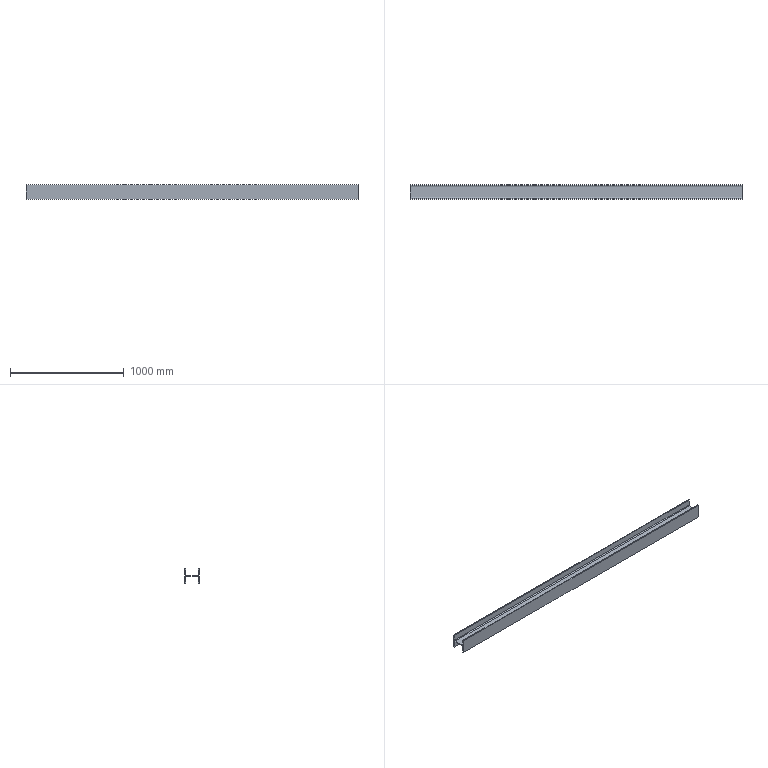Part | STEP file | 04-H125X125X6.5X9_default<machining> | 1 solid | 18 faces | box 2916 x 125 x 125 mm | volume 8749277 mm3 | plane 14 | cylinder 4 | commonest cylinder face diameters 16 x4
STEP:
#1=CARTESIAN_POINT('',(0.,0.,0.));
#2=DIRECTION('',(0.,0.,1.));
#3=DIRECTION('',(1.,0.,0.));
#4=AXIS2_PLACEMENT_3D('',#1,#2,#3);
#5=CARTESIAN_POINT('',(0.,62.5,62.5));
#6=VERTEX_POINT('',#5);
#7=CARTESIAN_POINT('',(0.,53.5,62.5));
#8=VERTEX_POINT('',#7);
#9=CARTESIAN_POINT('',(0.,62.5,62.5));
#10=DIRECTION('',(0.,-1.,0.));
#11=VECTOR('',#10,1.);
#12=LINE('',#9,#11);
#13=CARTESIAN_POINT('',(2916.,62.5,62.5));
#14=DIRECTION('',(0.,0.,-1.));
#15=DIRECTION('',(-1.,0.,0.));
#16=AXIS2_PLACEMENT_3D('',#13,#14,#15);
#17=PLANE('',#16);
#18=CARTESIAN_POINT('',(2916.,0.));
#19=DIRECTION('',(0.,-1.));
#20=VECTOR('',#19,1.);
#21=LINE('',#18,#20);
#22=(GEOMETRIC_REPRESENTATION_CONTEXT(2)PARAMETRIC_REPRESENTATION_CONTEXT()REPRESENTATION_CONTEXT('',''));
#23=DEFINITIONAL_REPRESENTATION('',(#21),#22);
#24=PCURVE('',#17,#23);
#25=CARTESIAN_POINT('',(0.,45.5,11.25));
#26=DIRECTION('',(1.,0.,0.));
#27=DIRECTION('',(0.,0.,-1.));
#28=AXIS2_PLACEMENT_3D('',#25,#26,#27);
#29=PLANE('',#28);
#30=CARTESIAN_POINT('',(-51.25,17.));
#31=DIRECTION('',(0.,-1.));
#32=VECTOR('',#31,1.);
#33=LINE('',#30,#32);
#34=(GEOMETRIC_REPRESENTATION_CONTEXT(2)PARAMETRIC_REPRESENTATION_CONTEXT()REPRESENTATION_CONTEXT('',''));
#35=DEFINITIONAL_REPRESENTATION('',(#33),#34);
#36=PCURVE('',#29,#35);
#37=SURFACE_CURVE('',#12,(#24,#36),.PCURVE_S1.);
#38=EDGE_CURVE('',#6,#8,#37,.T.);
#39=ORIENTED_EDGE('',*,*,#38,.T.);
#40=CARTESIAN_POINT('',(2916.,53.5,62.5));
#41=VERTEX_POINT('',#40);
#42=CARTESIAN_POINT('',(2916.,53.5,62.5));
#43=DIRECTION('',(-1.,0.,0.));
#44=VECTOR('',#43,1.);
#45=LINE('',#42,#44);
#46=CARTESIAN_POINT('',(0.,-9.));
#47=DIRECTION('',(1.,0.));
#48=VECTOR('',#47,1.);
#49=LINE('',#46,#48);
#50=(GEOMETRIC_REPRESENTATION_CONTEXT(2)PARAMETRIC_REPRESENTATION_CONTEXT()REPRESENTATION_CONTEXT('',''));
#51=DEFINITIONAL_REPRESENTATION('',(#49),#50);
#52=PCURVE('',#17,#51);
#53=CARTESIAN_POINT('',(2916.,53.5,62.5));
#54=DIRECTION('',(0.,1.,0.));
#55=DIRECTION('',(0.,0.,1.));
#56=AXIS2_PLACEMENT_3D('',#53,#54,#55);
#57=PLANE('',#56);
#58=CARTESIAN_POINT('',(0.,0.));
#59=DIRECTION('',(0.,-1.));
#60=VECTOR('',#59,1.);
#61=LINE('',#58,#60);
#62=(GEOMETRIC_REPRESENTATION_CONTEXT(2)PARAMETRIC_REPRESENTATION_CONTEXT()REPRESENTATION_CONTEXT('',''));
#63=DEFINITIONAL_REPRESENTATION('',(#61),#62);
#64=PCURVE('',#57,#63);
#65=SURFACE_CURVE('',#45,(#52,#64),.PCURVE_S1.);
#66=EDGE_CURVE('',#41,#8,#65,.T.);
#67=ORIENTED_EDGE('',*,*,#66,.F.);
#68=CARTESIAN_POINT('',(2916.,62.5,62.5));
#69=VERTEX_POINT('',#68);
#70=CARTESIAN_POINT('',(2916.,62.5,62.5));
#71=DIRECTION('',(0.,-1.,0.));
#72=VECTOR('',#71,1.);
#73=LINE('',#70,#72);
#74=CARTESIAN_POINT('',(0.,0.));
#75=DIRECTION('',(0.,-1.));
#76=VECTOR('',#75,1.);
#77=LINE('',#74,#76);
#78=(GEOMETRIC_REPRESENTATION_CONTEXT(2)PARAMETRIC_REPRESENTATION_CONTEXT()REPRESENTATION_CONTEXT('',''));
#79=DEFINITIONAL_REPRESENTATION('',(#77),#78);
#80=PCURVE('',#17,#79);
#81=CARTESIAN_POINT('',(2916.,45.5,11.25));
#82=DIRECTION('',(1.,0.,0.));
#83=DIRECTION('',(0.,0.,-1.));
#84=AXIS2_PLACEMENT_3D('',#81,#82,#83);
#85=PLANE('',#84);
#86=CARTESIAN_POINT('',(-51.25,17.));
#87=DIRECTION('',(0.,-1.));
#88=VECTOR('',#87,1.);
#89=LINE('',#86,#88);
#90=(GEOMETRIC_REPRESENTATION_CONTEXT(2)PARAMETRIC_REPRESENTATION_CONTEXT()REPRESENTATION_CONTEXT('',''));
#91=DEFINITIONAL_REPRESENTATION('',(#89),#90);
#92=PCURVE('',#85,#91);
#93=SURFACE_CURVE('',#73,(#80,#92),.PCURVE_S1.);
#94=EDGE_CURVE('',#69,#41,#93,.T.);
#95=ORIENTED_EDGE('',*,*,#94,.F.);
#96=CARTESIAN_POINT('',(2916.,62.5,62.5));
#97=DIRECTION('',(-1.,0.,0.));
#98=VECTOR('',#97,1.);
#99=LINE('',#96,#98);
#100=CARTESIAN_POINT('',(0.,0.));
#101=DIRECTION('',(1.,0.));
#102=VECTOR('',#101,1.);
#103=LINE('',#100,#102);
#104=(GEOMETRIC_REPRESENTATION_CONTEXT(2)PARAMETRIC_REPRESENTATION_CONTEXT()REPRESENTATION_CONTEXT('',''));
#105=DEFINITIONAL_REPRESENTATION('',(#103),#104);
#106=PCURVE('',#17,#105);
#107=CARTESIAN_POINT('',(2916.,62.5,-62.5));
#108=DIRECTION('',(0.,-1.,0.));
#109=DIRECTION('',(0.,0.,-1.));
#110=AXIS2_PLACEMENT_3D('',#107,#108,#109);
#111=PLANE('',#110);
#112=CARTESIAN_POINT('',(-125.,0.));
#113=DIRECTION('',(0.,-1.));
#114=VECTOR('',#113,1.);
#115=LINE('',#112,#114);
#116=(GEOMETRIC_REPRESENTATION_CONTEXT(2)PARAMETRIC_REPRESENTATION_CONTEXT()REPRESENTATION_CONTEXT('',''));
#117=DEFINITIONAL_REPRESENTATION('',(#115),#116);
#118=PCURVE('',#111,#117);
#119=SURFACE_CURVE('',#99,(#106,#118),.PCURVE_S1.);
#120=EDGE_CURVE('',#69,#6,#119,.T.);
#121=ORIENTED_EDGE('',*,*,#120,.T.);
#122=EDGE_LOOP('',(#39,#67,#95,#121));
#123=FACE_BOUND('',#122,.T.);
#124=ADVANCED_FACE('',(#123),#17,.F.);
#125=CARTESIAN_POINT('',(0.,53.5,11.25));
#126=VERTEX_POINT('',#125);
#127=CARTESIAN_POINT('',(0.,53.5,62.5));
#128=DIRECTION('',(0.,0.,-1.));
#129=VECTOR('',#128,1.);
#130=LINE('',#127,#129);
#131=CARTESIAN_POINT('',(0.,-2916.));
#132=DIRECTION('',(-1.,0.));
#133=VECTOR('',#132,1.);
#134=LINE('',#131,#133);
#135=(GEOMETRIC_REPRESENTATION_CONTEXT(2)PARAMETRIC_REPRESENTATION_CONTEXT()REPRESENTATION_CONTEXT('',''));
#136=DEFINITIONAL_REPRESENTATION('',(#134),#135);
#137=PCURVE('',#57,#136);
#138=CARTESIAN_POINT('',(-51.25,8.));
#139=DIRECTION('',(1.,0.));
#140=VECTOR('',#139,1.);
#141=LINE('',#138,#140);
#142=(GEOMETRIC_REPRESENTATION_CONTEXT(2)PARAMETRIC_REPRESENTATION_CONTEXT()REPRESENTATION_CONTEXT('',''));
#143=DEFINITIONAL_REPRESENTATION('',(#141),#142);
#144=PCURVE('',#29,#143);
#145=SURFACE_CURVE('',#130,(#137,#144),.PCURVE_S1.);
#146=EDGE_CURVE('',#8,#126,#145,.T.);
#147=ORIENTED_EDGE('',*,*,#146,.T.);
#148=CARTESIAN_POINT('',(2916.,53.5,11.25));
#149=VERTEX_POINT('',#148);
#150=CARTESIAN_POINT('',(2916.,53.5,11.25));
#151=DIRECTION('',(-1.,0.,0.));
#152=VECTOR('',#151,1.);
#153=LINE('',#150,#152);
#154=CARTESIAN_POINT('',(-51.25,0.));
#155=DIRECTION('',(0.,-1.));
#156=VECTOR('',#155,1.);
#157=LINE('',#154,#156);
#158=(GEOMETRIC_REPRESENTATION_CONTEXT(2)PARAMETRIC_REPRESENTATION_CONTEXT()REPRESENTATION_CONTEXT('',''));
#159=DEFINITIONAL_REPRESENTATION('',(#157),#158);
#160=PCURVE('',#57,#159);
#161=CARTESIAN_POINT('',(2916.,45.5,11.25));
#162=DIRECTION('',(-1.,0.,0.));
#163=DIRECTION('',(0.,0.,1.));
#164=AXIS2_PLACEMENT_3D('',#161,#162,#163);
#165=CYLINDRICAL_SURFACE('',#164,8.);
#166=CARTESIAN_POINT('',(1.571,0.));
#167=DIRECTION('',(0.,1.));
#168=VECTOR('',#167,1.);
#169=LINE('',#166,#168);
#170=(GEOMETRIC_REPRESENTATION_CONTEXT(2)PARAMETRIC_REPRESENTATION_CONTEXT()REPRESENTATION_CONTEXT('',''));
#171=DEFINITIONAL_REPRESENTATION('',(#169),#170);
#172=PCURVE('',#165,#171);
#173=SURFACE_CURVE('',#153,(#160,#172),.PCURVE_S1.);
#174=EDGE_CURVE('',#149,#126,#173,.T.);
#175=ORIENTED_EDGE('',*,*,#174,.F.);
#176=CARTESIAN_POINT('',(2916.,53.5,62.5));
#177=DIRECTION('',(0.,0.,-1.));
#178=VECTOR('',#177,1.);
#179=LINE('',#176,#178);
#180=CARTESIAN_POINT('',(0.,0.));
#181=DIRECTION('',(-1.,0.));
#182=VECTOR('',#181,1.);
#183=LINE('',#180,#182);
#184=(GEOMETRIC_REPRESENTATION_CONTEXT(2)PARAMETRIC_REPRESENTATION_CONTEXT()REPRESENTATION_CONTEXT('',''));
#185=DEFINITIONAL_REPRESENTATION('',(#183),#184);
#186=PCURVE('',#57,#185);
#187=CARTESIAN_POINT('',(-51.25,8.));
#188=DIRECTION('',(1.,0.));
#189=VECTOR('',#188,1.);
#190=LINE('',#187,#189);
#191=(GEOMETRIC_REPRESENTATION_CONTEXT(2)PARAMETRIC_REPRESENTATION_CONTEXT()REPRESENTATION_CONTEXT('',''));
#192=DEFINITIONAL_REPRESENTATION('',(#190),#191);
#193=PCURVE('',#85,#192);
#194=SURFACE_CURVE('',#179,(#186,#193),.PCURVE_S1.);
#195=EDGE_CURVE('',#41,#149,#194,.T.);
#196=ORIENTED_EDGE('',*,*,#195,.F.);
#197=ORIENTED_EDGE('',*,*,#66,.T.);
#198=EDGE_LOOP('',(#147,#175,#196,#197));
#199=FACE_BOUND('',#198,.T.);
#200=ADVANCED_FACE('',(#199),#57,.F.);
#201=ORIENTED_EDGE('',*,*,#174,.F.);
#202=CARTESIAN_POINT('',(2916.,45.5,3.25));
#203=VERTEX_POINT('',#202);
#204=CARTESIAN_POINT('',(2916.,45.5,11.25));
#205=DIRECTION('',(-1.,0.,0.));
#206=DIRECTION('',(0.,0.,-1.));
#207=AXIS2_PLACEMENT_3D('',#204,#205,#206);
#208=CIRCLE('',#207,8.);
#209=CARTESIAN_POINT('',(-3.142,0.));
#210=DIRECTION('',(1.,0.));
#211=VECTOR('',#210,1.);
#212=LINE('',#209,#211);
#213=(GEOMETRIC_REPRESENTATION_CONTEXT(2)PARAMETRIC_REPRESENTATION_CONTEXT()REPRESENTATION_CONTEXT('',''));
#214=DEFINITIONAL_REPRESENTATION('',(#212),#213);
#215=PCURVE('',#165,#214);
#216=CARTESIAN_POINT('',(8.,0.));
#217=CARTESIAN_POINT('',(8.,-13.856));
#218=CARTESIAN_POINT('',(-4.,-6.928));
#219=CARTESIAN_POINT('',(-16.,0.));
#220=CARTESIAN_POINT('',(-4.,6.928));
#221=CARTESIAN_POINT('',(8.,13.856));
#222=CARTESIAN_POINT('',(8.,0.));
#223=(BOUNDED_CURVE()B_SPLINE_CURVE(2,(#216,#217,#218,#219,#220,#221,#222),.UNSPECIFIED.,.T.,.F.)B_SPLINE_CURVE_WITH_KNOTS((1,2,2,2,2,1),(-2.094,0.,2.094,4.189,6.283,8.378),.UNSPECIFIED.)CURVE()GEOMETRIC_REPRESENTATION_ITEM()RATIONAL_B_SPLINE_CURVE((1.,0.5,1.,0.5,1.,0.5,1.))REPRESENTATION_ITEM(''));
#224=(GEOMETRIC_REPRESENTATION_CONTEXT(2)PARAMETRIC_REPRESENTATION_CONTEXT()REPRESENTATION_CONTEXT('',''));
#225=DEFINITIONAL_REPRESENTATION('',(#223),#224);
#226=PCURVE('',#85,#225);
#227=SURFACE_CURVE('',#208,(#215,#226),.PCURVE_S1.);
#228=EDGE_CURVE('',#149,#203,#227,.T.);
#229=ORIENTED_EDGE('',*,*,#228,.T.);
#230=CARTESIAN_POINT('',(0.,45.5,3.25));
#231=VERTEX_POINT('',#230);
#232=CARTESIAN_POINT('',(2916.,45.5,3.25));
#233=DIRECTION('',(-1.,0.,0.));
#234=VECTOR('',#233,1.);
#235=LINE('',#232,#234);
#236=CARTESIAN_POINT('',(3.142,0.));
#237=DIRECTION('',(0.,1.));
#238=VECTOR('',#237,1.);
#239=LINE('',#236,#238);
#240=(GEOMETRIC_REPRESENTATION_CONTEXT(2)PARAMETRIC_REPRESENTATION_CONTEXT()REPRESENTATION_CONTEXT('',''));
#241=DEFINITIONAL_REPRESENTATION('',(#239),#240);
#242=PCURVE('',#165,#241);
#243=CARTESIAN_POINT('',(2916.,45.5,3.25));
#244=DIRECTION('',(0.,0.,-1.));
#245=DIRECTION('',(-1.,0.,0.));
#246=AXIS2_PLACEMENT_3D('',#243,#244,#245);
#247=PLANE('',#246);
#248=CARTESIAN_POINT('',(0.,0.));
#249=DIRECTION('',(1.,0.));
#250=VECTOR('',#249,1.);
#251=LINE('',#248,#250);
#252=(GEOMETRIC_REPRESENTATION_CONTEXT(2)PARAMETRIC_REPRESENTATION_CONTEXT()REPRESENTATION_CONTEXT('',''));
#253=DEFINITIONAL_REPRESENTATION('',(#251),#252);
#254=PCURVE('',#247,#253);
#255=SURFACE_CURVE('',#235,(#242,#254),.PCURVE_S1.);
#256=EDGE_CURVE('',#203,#231,#255,.T.);
#257=ORIENTED_EDGE('',*,*,#256,.T.);
#258=CARTESIAN_POINT('',(0.,45.5,11.25));
#259=DIRECTION('',(-1.,0.,0.));
#260=DIRECTION('',(0.,0.,-1.));
#261=AXIS2_PLACEMENT_3D('',#258,#259,#260);
#262=CIRCLE('',#261,8.);
#263=CARTESIAN_POINT('',(-3.142,2916.));
#264=DIRECTION('',(1.,0.));
#265=VECTOR('',#264,1.);
#266=LINE('',#263,#265);
#267=(GEOMETRIC_REPRESENTATION_CONTEXT(2)PARAMETRIC_REPRESENTATION_CONTEXT()REPRESENTATION_CONTEXT('',''));
#268=DEFINITIONAL_REPRESENTATION('',(#266),#267);
#269=PCURVE('',#165,#268);
#270=CARTESIAN_POINT('',(8.,0.));
#271=CARTESIAN_POINT('',(8.,-13.856));
#272=CARTESIAN_POINT('',(-4.,-6.928));
#273=CARTESIAN_POINT('',(-16.,0.));
#274=CARTESIAN_POINT('',(-4.,6.928));
#275=CARTESIAN_POINT('',(8.,13.856));
#276=CARTESIAN_POINT('',(8.,0.));
#277=(BOUNDED_CURVE()B_SPLINE_CURVE(2,(#270,#271,#272,#273,#274,#275,#276),.UNSPECIFIED.,.T.,.F.)B_SPLINE_CURVE_WITH_KNOTS((1,2,2,2,2,1),(-2.094,0.,2.094,4.189,6.283,8.378),.UNSPECIFIED.)CURVE()GEOMETRIC_REPRESENTATION_ITEM()RATIONAL_B_SPLINE_CURVE((1.,0.5,1.,0.5,1.,0.5,1.))REPRESENTATION_ITEM(''));
#278=(GEOMETRIC_REPRESENTATION_CONTEXT(2)PARAMETRIC_REPRESENTATION_CONTEXT()REPRESENTATION_CONTEXT('',''));
#279=DEFINITIONAL_REPRESENTATION('',(#277),#278);
#280=PCURVE('',#29,#279);
#281=SURFACE_CURVE('',#262,(#269,#280),.PCURVE_S1.);
#282=EDGE_CURVE('',#126,#231,#281,.T.);
#283=ORIENTED_EDGE('',*,*,#282,.F.);
#284=EDGE_LOOP('',(#201,#229,#257,#283));
#285=FACE_BOUND('',#284,.F.);
#286=ADVANCED_FACE('',(#285),#165,.F.);
#287=CARTESIAN_POINT('',(0.,-45.5,3.25));
#288=VERTEX_POINT('',#287);
#289=CARTESIAN_POINT('',(0.,45.5,3.25));
#290=DIRECTION('',(0.,-1.,0.));
#291=VECTOR('',#290,1.);
#292=LINE('',#289,#291);
#293=CARTESIAN_POINT('',(2916.,0.));
#294=DIRECTION('',(0.,-1.));
#295=VECTOR('',#294,1.);
#296=LINE('',#293,#295);
#297=(GEOMETRIC_REPRESENTATION_CONTEXT(2)PARAMETRIC_REPRESENTATION_CONTEXT()REPRESENTATION_CONTEXT('',''));
#298=DEFINITIONAL_REPRESENTATION('',(#296),#297);
#299=PCURVE('',#247,#298);
#300=CARTESIAN_POINT('',(8.,0.));
#301=DIRECTION('',(0.,-1.));
#302=VECTOR('',#301,1.);
#303=LINE('',#300,#302);
#304=(GEOMETRIC_REPRESENTATION_CONTEXT(2)PARAMETRIC_REPRESENTATION_CONTEXT()REPRESENTATION_CONTEXT('',''));
#305=DEFINITIONAL_REPRESENTATION('',(#303),#304);
#306=PCURVE('',#29,#305);
#307=SURFACE_CURVE('',#292,(#299,#306),.PCURVE_S1.);
#308=EDGE_CURVE('',#231,#288,#307,.T.);
#309=ORIENTED_EDGE('',*,*,#308,.T.);
#310=CARTESIAN_POINT('',(2916.,-45.5,3.25));
#311=VERTEX_POINT('',#310);
#312=CARTESIAN_POINT('',(2916.,-45.5,3.25));
#313=DIRECTION('',(-1.,0.,0.));
#314=VECTOR('',#313,1.);
#315=LINE('',#312,#314);
#316=CARTESIAN_POINT('',(0.,-91.));
#317=DIRECTION('',(1.,0.));
#318=VECTOR('',#317,1.);
#319=LINE('',#316,#318);
#320=(GEOMETRIC_REPRESENTATION_CONTEXT(2)PARAMETRIC_REPRESENTATION_CONTEXT()REPRESENTATION_CONTEXT('',''));
#321=DEFINITIONAL_REPRESENTATION('',(#319),#320);
#322=PCURVE('',#247,#321);
#323=CARTESIAN_POINT('',(2916.,-45.5,11.25));
#324=DIRECTION('',(-1.,0.,0.));
#325=DIRECTION('',(0.,0.,1.));
#326=AXIS2_PLACEMENT_3D('',#323,#324,#325);
#327=CYLINDRICAL_SURFACE('',#326,8.);
#328=CARTESIAN_POINT('',(3.142,0.));
#329=DIRECTION('',(0.,1.));
#330=VECTOR('',#329,1.);
#331=LINE('',#328,#330);
#332=(GEOMETRIC_REPRESENTATION_CONTEXT(2)PARAMETRIC_REPRESENTATION_CONTEXT()REPRESENTATION_CONTEXT('',''));
#333=DEFINITIONAL_REPRESENTATION('',(#331),#332);
#334=PCURVE('',#327,#333);
#335=SURFACE_CURVE('',#315,(#322,#334),.PCURVE_S1.);
#336=EDGE_CURVE('',#311,#288,#335,.T.);
#337=ORIENTED_EDGE('',*,*,#336,.F.);
#338=CARTESIAN_POINT('',(2916.,45.5,3.25));
#339=DIRECTION('',(0.,-1.,0.));
#340=VECTOR('',#339,1.);
#341=LINE('',#338,#340);
#342=CARTESIAN_POINT('',(0.,0.));
#343=DIRECTION('',(0.,-1.));
#344=VECTOR('',#343,1.);
#345=LINE('',#342,#344);
#346=(GEOMETRIC_REPRESENTATION_CONTEXT(2)PARAMETRIC_REPRESENTATION_CONTEXT()REPRESENTATION_CONTEXT('',''));
#347=DEFINITIONAL_REPRESENTATION('',(#345),#346);
#348=PCURVE('',#247,#347);
#349=CARTESIAN_POINT('',(8.,0.));
#350=DIRECTION('',(0.,-1.));
#351=VECTOR('',#350,1.);
#352=LINE('',#349,#351);
#353=(GEOMETRIC_REPRESENTATION_CONTEXT(2)PARAMETRIC_REPRESENTATION_CONTEXT()REPRESENTATION_CONTEXT('',''));
#354=DEFINITIONAL_REPRESENTATION('',(#352),#353);
#355=PCURVE('',#85,#354);
#356=SURFACE_CURVE('',#341,(#348,#355),.PCURVE_S1.);
#357=EDGE_CURVE('',#203,#311,#356,.T.);
#358=ORIENTED_EDGE('',*,*,#357,.F.);
#359=ORIENTED_EDGE('',*,*,#256,.T.);
#360=EDGE_LOOP('',(#309,#337,#358,#359));
#361=FACE_BOUND('',#360,.T.);
#362=ADVANCED_FACE('',(#361),#247,.F.);
#363=ORIENTED_EDGE('',*,*,#336,.F.);
#364=CARTESIAN_POINT('',(2916.,-53.5,11.25));
#365=VERTEX_POINT('',#364);
#366=CARTESIAN_POINT('',(2916.,-45.5,11.25));
#367=DIRECTION('',(-1.,0.,0.));
#368=DIRECTION('',(0.,0.,-1.));
#369=AXIS2_PLACEMENT_3D('',#366,#367,#368);
#370=CIRCLE('',#369,8.);
#371=CARTESIAN_POINT('',(3.142,0.));
#372=DIRECTION('',(1.,0.));
#373=VECTOR('',#372,1.);
#374=LINE('',#371,#373);
#375=(GEOMETRIC_REPRESENTATION_CONTEXT(2)PARAMETRIC_REPRESENTATION_CONTEXT()REPRESENTATION_CONTEXT('',''));
#376=DEFINITIONAL_REPRESENTATION('',(#374),#375);
#377=PCURVE('',#327,#376);
#378=CARTESIAN_POINT('',(8.,-91.));
#379=CARTESIAN_POINT('',(8.,-104.856));
#380=CARTESIAN_POINT('',(-4.,-97.928));
#381=CARTESIAN_POINT('',(-16.,-91.));
#382=CARTESIAN_POINT('',(-4.,-84.072));
#383=CARTESIAN_POINT('',(8.,-77.144));
#384=CARTESIAN_POINT('',(8.,-91.));
#385=(BOUNDED_CURVE()B_SPLINE_CURVE(2,(#378,#379,#380,#381,#382,#383,#384),.UNSPECIFIED.,.T.,.F.)B_SPLINE_CURVE_WITH_KNOTS((1,2,2,2,2,1),(-2.094,0.,2.094,4.189,6.283,8.378),.UNSPECIFIED.)CURVE()GEOMETRIC_REPRESENTATION_ITEM()RATIONAL_B_SPLINE_CURVE((1.,0.5,1.,0.5,1.,0.5,1.))REPRESENTATION_ITEM(''));
#386=(GEOMETRIC_REPRESENTATION_CONTEXT(2)PARAMETRIC_REPRESENTATION_CONTEXT()REPRESENTATION_CONTEXT('',''));
#387=DEFINITIONAL_REPRESENTATION('',(#385),#386);
#388=PCURVE('',#85,#387);
#389=SURFACE_CURVE('',#370,(#377,#388),.PCURVE_S1.);
#390=EDGE_CURVE('',#311,#365,#389,.T.);
#391=ORIENTED_EDGE('',*,*,#390,.T.);
#392=CARTESIAN_POINT('',(0.,-53.5,11.25));
#393=VERTEX_POINT('',#392);
#394=CARTESIAN_POINT('',(2916.,-53.5,11.25));
#395=DIRECTION('',(-1.,0.,0.));
#396=VECTOR('',#395,1.);
#397=LINE('',#394,#396);
#398=CARTESIAN_POINT('',(4.712,0.));
#399=DIRECTION('',(0.,1.));
#400=VECTOR('',#399,1.);
#401=LINE('',#398,#400);
#402=(GEOMETRIC_REPRESENTATION_CONTEXT(2)PARAMETRIC_REPRESENTATION_CONTEXT()REPRESENTATION_CONTEXT('',''));
#403=DEFINITIONAL_REPRESENTATION('',(#401),#402);
#404=PCURVE('',#327,#403);
#405=CARTESIAN_POINT('',(2916.,-53.5,62.5));
#406=DIRECTION('',(0.,-1.,0.));
#407=DIRECTION('',(0.,0.,-1.));
#408=AXIS2_PLACEMENT_3D('',#405,#406,#407);
#409=PLANE('',#408);
#410=CARTESIAN_POINT('',(51.25,0.));
#411=DIRECTION('',(0.,-1.));
#412=VECTOR('',#411,1.);
#413=LINE('',#410,#412);
#414=(GEOMETRIC_REPRESENTATION_CONTEXT(2)PARAMETRIC_REPRESENTATION_CONTEXT()REPRESENTATION_CONTEXT('',''));
#415=DEFINITIONAL_REPRESENTATION('',(#413),#414);
#416=PCURVE('',#409,#415);
#417=SURFACE_CURVE('',#397,(#404,#416),.PCURVE_S1.);
#418=EDGE_CURVE('',#365,#393,#417,.T.);
#419=ORIENTED_EDGE('',*,*,#418,.T.);
#420=CARTESIAN_POINT('',(0.,-45.5,11.25));
#421=DIRECTION('',(-1.,0.,0.));
#422=DIRECTION('',(0.,0.,-1.));
#423=AXIS2_PLACEMENT_3D('',#420,#421,#422);
#424=CIRCLE('',#423,8.);
#425=CARTESIAN_POINT('',(3.142,2916.));
#426=DIRECTION('',(1.,0.));
#427=VECTOR('',#426,1.);
#428=LINE('',#425,#427);
#429=(GEOMETRIC_REPRESENTATION_CONTEXT(2)PARAMETRIC_REPRESENTATION_CONTEXT()REPRESENTATION_CONTEXT('',''));
#430=DEFINITIONAL_REPRESENTATION('',(#428),#429);
#431=PCURVE('',#327,#430);
#432=CARTESIAN_POINT('',(8.,-91.));
#433=CARTESIAN_POINT('',(8.,-104.856));
#434=CARTESIAN_POINT('',(-4.,-97.928));
#435=CARTESIAN_POINT('',(-16.,-91.));
#436=CARTESIAN_POINT('',(-4.,-84.072));
#437=CARTESIAN_POINT('',(8.,-77.144));
#438=CARTESIAN_POINT('',(8.,-91.));
#439=(BOUNDED_CURVE()B_SPLINE_CURVE(2,(#432,#433,#434,#435,#436,#437,#438),.UNSPECIFIED.,.T.,.F.)B_SPLINE_CURVE_WITH_KNOTS((1,2,2,2,2,1),(-2.094,0.,2.094,4.189,6.283,8.378),.UNSPECIFIED.)CURVE()GEOMETRIC_REPRESENTATION_ITEM()RATIONAL_B_SPLINE_CURVE((1.,0.5,1.,0.5,1.,0.5,1.))REPRESENTATION_ITEM(''));
#440=(GEOMETRIC_REPRESENTATION_CONTEXT(2)PARAMETRIC_REPRESENTATION_CONTEXT()REPRESENTATION_CONTEXT('',''));
#441=DEFINITIONAL_REPRESENTATION('',(#439),#440);
#442=PCURVE('',#29,#441);
#443=SURFACE_CURVE('',#424,(#431,#442),.PCURVE_S1.);
#444=EDGE_CURVE('',#288,#393,#443,.T.);
#445=ORIENTED_EDGE('',*,*,#444,.F.);
#446=EDGE_LOOP('',(#363,#391,#419,#445));
#447=FACE_BOUND('',#446,.F.);
#448=ADVANCED_FACE('',(#447),#327,.F.);
#449=CARTESIAN_POINT('',(0.,-53.5,62.5));
#450=VERTEX_POINT('',#449);
#451=CARTESIAN_POINT('',(0.,-53.5,62.5));
#452=DIRECTION('',(0.,0.,1.));
#453=VECTOR('',#452,1.);
#454=LINE('',#451,#453);
#455=CARTESIAN_POINT('',(0.,-2916.));
#456=DIRECTION('',(-1.,0.));
#457=VECTOR('',#456,1.);
#458=LINE('',#455,#457);
#459=(GEOMETRIC_REPRESENTATION_CONTEXT(2)PARAMETRIC_REPRESENTATION_CONTEXT()REPRESENTATION_CONTEXT('',''));
#460=DEFINITIONAL_REPRESENTATION('',(#458),#459);
#461=PCURVE('',#409,#460);
#462=CARTESIAN_POINT('',(-51.25,-99.));
#463=DIRECTION('',(-1.,0.));
#464=VECTOR('',#463,1.);
#465=LINE('',#462,#464);
#466=(GEOMETRIC_REPRESENTATION_CONTEXT(2)PARAMETRIC_REPRESENTATION_CONTEXT()REPRESENTATION_CONTEXT('',''));
#467=DEFINITIONAL_REPRESENTATION('',(#465),#466);
#468=PCURVE('',#29,#467);
#469=SURFACE_CURVE('',#454,(#461,#468),.PCURVE_S1.);
#470=EDGE_CURVE('',#393,#450,#469,.T.);
#471=ORIENTED_EDGE('',*,*,#470,.T.);
#472=CARTESIAN_POINT('',(2916.,-53.5,62.5));
#473=VERTEX_POINT('',#472);
#474=CARTESIAN_POINT('',(2916.,-53.5,62.5));
#475=DIRECTION('',(-1.,0.,0.));
#476=VECTOR('',#475,1.);
#477=LINE('',#474,#476);
#478=CARTESIAN_POINT('',(0.,0.));
#479=DIRECTION('',(0.,-1.));
#480=VECTOR('',#479,1.);
#481=LINE('',#478,#480);
#482=(GEOMETRIC_REPRESENTATION_CONTEXT(2)PARAMETRIC_REPRESENTATION_CONTEXT()REPRESENTATION_CONTEXT('',''));
#483=DEFINITIONAL_REPRESENTATION('',(#481),#482);
#484=PCURVE('',#409,#483);
#485=CARTESIAN_POINT('',(2916.,-62.5,62.5));
#486=DIRECTION('',(0.,0.,-1.));
#487=DIRECTION('',(0.,1.,0.));
#488=AXIS2_PLACEMENT_3D('',#485,#486,#487);
#489=PLANE('',#488);
#490=CARTESIAN_POINT('',(9.,0.));
#491=DIRECTION('',(0.,-1.));
#492=VECTOR('',#491,1.);
#493=LINE('',#490,#492);
#494=(GEOMETRIC_REPRESENTATION_CONTEXT(2)PARAMETRIC_REPRESENTATION_CONTEXT()REPRESENTATION_CONTEXT('',''));
#495=DEFINITIONAL_REPRESENTATION('',(#493),#494);
#496=PCURVE('',#489,#495);
#497=SURFACE_CURVE('',#477,(#484,#496),.PCURVE_S1.);
#498=EDGE_CURVE('',#473,#450,#497,.T.);
#499=ORIENTED_EDGE('',*,*,#498,.F.);
#500=CARTESIAN_POINT('',(2916.,-53.5,62.5));
#501=DIRECTION('',(0.,0.,1.));
#502=VECTOR('',#501,1.);
#503=LINE('',#500,#502);
#504=CARTESIAN_POINT('',(0.,0.));
#505=DIRECTION('',(-1.,0.));
#506=VECTOR('',#505,1.);
#507=LINE('',#504,#506);
#508=(GEOMETRIC_REPRESENTATION_CONTEXT(2)PARAMETRIC_REPRESENTATION_CONTEXT()REPRESENTATION_CONTEXT('',''));
#509=DEFINITIONAL_REPRESENTATION('',(#507),#508);
#510=PCURVE('',#409,#509);
#511=CARTESIAN_POINT('',(-51.25,-99.));
#512=DIRECTION('',(-1.,0.));
#513=VECTOR('',#512,1.);
#514=LINE('',#511,#513);
#515=(GEOMETRIC_REPRESENTATION_CONTEXT(2)PARAMETRIC_REPRESENTATION_CONTEXT()REPRESENTATION_CONTEXT('',''));
#516=DEFINITIONAL_REPRESENTATION('',(#514),#515);
#517=PCURVE('',#85,#516);
#518=SURFACE_CURVE('',#503,(#510,#517),.PCURVE_S1.);
#519=EDGE_CURVE('',#365,#473,#518,.T.);
#520=ORIENTED_EDGE('',*,*,#519,.F.);
#521=ORIENTED_EDGE('',*,*,#418,.T.);
#522=EDGE_LOOP('',(#471,#499,#520,#521));
#523=FACE_BOUND('',#522,.T.);
#524=ADVANCED_FACE('',(#523),#409,.F.);
#525=CARTESIAN_POINT('',(0.,-62.5,62.5));
#526=VERTEX_POINT('',#525);
#527=CARTESIAN_POINT('',(0.,-62.5,62.5));
#528=DIRECTION('',(0.,-1.,0.));
#529=VECTOR('',#528,1.);
#530=LINE('',#527,#529);
#531=CARTESIAN_POINT('',(0.,-2916.));
#532=DIRECTION('',(-1.,0.));
#533=VECTOR('',#532,1.);
#534=LINE('',#531,#533);
#535=(GEOMETRIC_REPRESENTATION_CONTEXT(2)PARAMETRIC_REPRESENTATION_CONTEXT()REPRESENTATION_CONTEXT('',''));
#536=DEFINITIONAL_REPRESENTATION('',(#534),#535);
#537=PCURVE('',#489,#536);
#538=CARTESIAN_POINT('',(-51.25,-108.));
#539=DIRECTION('',(0.,-1.));
#540=VECTOR('',#539,1.);
#541=LINE('',#538,#540);
#542=(GEOMETRIC_REPRESENTATION_CONTEXT(2)PARAMETRIC_REPRESENTATION_CONTEXT()REPRESENTATION_CONTEXT('',''));
#543=DEFINITIONAL_REPRESENTATION('',(#541),#542);
#544=PCURVE('',#29,#543);
#545=SURFACE_CURVE('',#530,(#537,#544),.PCURVE_S1.);
#546=EDGE_CURVE('',#450,#526,#545,.T.);
#547=ORIENTED_EDGE('',*,*,#546,.T.);
#548=CARTESIAN_POINT('',(2916.,-62.5,62.5));
#549=VERTEX_POINT('',#548);
#550=CARTESIAN_POINT('',(2916.,-62.5,62.5));
#551=DIRECTION('',(-1.,0.,0.));
#552=VECTOR('',#551,1.);
#553=LINE('',#550,#552);
#554=CARTESIAN_POINT('',(0.,0.));
#555=DIRECTION('',(0.,-1.));
#556=VECTOR('',#555,1.);
#557=LINE('',#554,#556);
#558=(GEOMETRIC_REPRESENTATION_CONTEXT(2)PARAMETRIC_REPRESENTATION_CONTEXT()REPRESENTATION_CONTEXT('',''));
#559=DEFINITIONAL_REPRESENTATION('',(#557),#558);
#560=PCURVE('',#489,#559);
#561=CARTESIAN_POINT('',(2916.,-62.5,-62.5));
#562=DIRECTION('',(0.,1.,0.));
#563=DIRECTION('',(0.,0.,1.));
#564=AXIS2_PLACEMENT_3D('',#561,#562,#563);
#565=PLANE('',#564);
#566=CARTESIAN_POINT('',(125.,0.));
#567=DIRECTION('',(0.,-1.));
#568=VECTOR('',#567,1.);
#569=LINE('',#566,#568);
#570=(GEOMETRIC_REPRESENTATION_CONTEXT(2)PARAMETRIC_REPRESENTATION_CONTEXT()REPRESENTATION_CONTEXT('',''));
#571=DEFINITIONAL_REPRESENTATION('',(#569),#570);
#572=PCURVE('',#565,#571);
#573=SURFACE_CURVE('',#553,(#560,#572),.PCURVE_S1.);
#574=EDGE_CURVE('',#549,#526,#573,.T.);
#575=ORIENTED_EDGE('',*,*,#574,.F.);
#576=CARTESIAN_POINT('',(2916.,-62.5,62.5));
#577=DIRECTION('',(0.,-1.,0.));
#578=VECTOR('',#577,1.);
#579=LINE('',#576,#578);
#580=CARTESIAN_POINT('',(0.,0.));
#581=DIRECTION('',(-1.,0.));
#582=VECTOR('',#581,1.);
#583=LINE('',#580,#582);
#584=(GEOMETRIC_REPRESENTATION_CONTEXT(2)PARAMETRIC_REPRESENTATION_CONTEXT()REPRESENTATION_CONTEXT('',''));
#585=DEFINITIONAL_REPRESENTATION('',(#583),#584);
#586=PCURVE('',#489,#585);
#587=CARTESIAN_POINT('',(-51.25,-108.));
#588=DIRECTION('',(0.,-1.));
#589=VECTOR('',#588,1.);
#590=LINE('',#587,#589);
#591=(GEOMETRIC_REPRESENTATION_CONTEXT(2)PARAMETRIC_REPRESENTATION_CONTEXT()REPRESENTATION_CONTEXT('',''));
#592=DEFINITIONAL_REPRESENTATION('',(#590),#591);
#593=PCURVE('',#85,#592);
#594=SURFACE_CURVE('',#579,(#586,#593),.PCURVE_S1.);
#595=EDGE_CURVE('',#473,#549,#594,.T.);
#596=ORIENTED_EDGE('',*,*,#595,.F.);
#597=ORIENTED_EDGE('',*,*,#498,.T.);
#598=EDGE_LOOP('',(#547,#575,#596,#597));
#599=FACE_BOUND('',#598,.T.);
#600=ADVANCED_FACE('',(#599),#489,.F.);
#601=CARTESIAN_POINT('',(0.,-62.5,-62.5));
#602=VERTEX_POINT('',#601);
#603=CARTESIAN_POINT('',(0.,-62.5,-62.5));
#604=DIRECTION('',(0.,0.,-1.));
#605=VECTOR('',#604,1.);
#606=LINE('',#603,#605);
#607=CARTESIAN_POINT('',(0.,-2916.));
#608=DIRECTION('',(-1.,0.));
#609=VECTOR('',#608,1.);
#610=LINE('',#607,#609);
#611=(GEOMETRIC_REPRESENTATION_CONTEXT(2)PARAMETRIC_REPRESENTATION_CONTEXT()REPRESENTATION_CONTEXT('',''));
#612=DEFINITIONAL_REPRESENTATION('',(#610),#611);
#613=PCURVE('',#565,#612);
#614=CARTESIAN_POINT('',(73.75,-108.));
#615=DIRECTION('',(1.,0.));
#616=VECTOR('',#615,1.);
#617=LINE('',#614,#616);
#618=(GEOMETRIC_REPRESENTATION_CONTEXT(2)PARAMETRIC_REPRESENTATION_CONTEXT()REPRESENTATION_CONTEXT('',''));
#619=DEFINITIONAL_REPRESENTATION('',(#617),#618);
#620=PCURVE('',#29,#619);
#621=SURFACE_CURVE('',#606,(#613,#620),.PCURVE_S1.);
#622=EDGE_CURVE('',#526,#602,#621,.T.);
#623=ORIENTED_EDGE('',*,*,#622,.T.);
#624=CARTESIAN_POINT('',(2916.,-62.5,-62.5));
#625=VERTEX_POINT('',#624);
#626=CARTESIAN_POINT('',(2916.,-62.5,-62.5));
#627=DIRECTION('',(-1.,0.,0.));
#628=VECTOR('',#627,1.);
#629=LINE('',#626,#628);
#630=CARTESIAN_POINT('',(0.,0.));
#631=DIRECTION('',(0.,-1.));
#632=VECTOR('',#631,1.);
#633=LINE('',#630,#632);
#634=(GEOMETRIC_REPRESENTATION_CONTEXT(2)PARAMETRIC_REPRESENTATION_CONTEXT()REPRESENTATION_CONTEXT('',''));
#635=DEFINITIONAL_REPRESENTATION('',(#633),#634);
#636=PCURVE('',#565,#635);
#637=CARTESIAN_POINT('',(2916.,-62.5,-62.5));
#638=DIRECTION('',(0.,0.,1.));
#639=DIRECTION('',(1.,0.,0.));
#640=AXIS2_PLACEMENT_3D('',#637,#638,#639);
#641=PLANE('',#640);
#642=CARTESIAN_POINT('',(0.,0.));
#643=DIRECTION('',(-1.,0.));
#644=VECTOR('',#643,1.);
#645=LINE('',#642,#644);
#646=(GEOMETRIC_REPRESENTATION_CONTEXT(2)PARAMETRIC_REPRESENTATION_CONTEXT()REPRESENTATION_CONTEXT('',''));
#647=DEFINITIONAL_REPRESENTATION('',(#645),#646);
#648=PCURVE('',#641,#647);
#649=SURFACE_CURVE('',#629,(#636,#648),.PCURVE_S1.);
#650=EDGE_CURVE('',#625,#602,#649,.T.);
#651=ORIENTED_EDGE('',*,*,#650,.F.);
#652=CARTESIAN_POINT('',(2916.,-62.5,-62.5));
#653=DIRECTION('',(0.,0.,-1.));
#654=VECTOR('',#653,1.);
#655=LINE('',#652,#654);
#656=CARTESIAN_POINT('',(0.,0.));
#657=DIRECTION('',(-1.,0.));
#658=VECTOR('',#657,1.);
#659=LINE('',#656,#658);
#660=(GEOMETRIC_REPRESENTATION_CONTEXT(2)PARAMETRIC_REPRESENTATION_CONTEXT()REPRESENTATION_CONTEXT('',''));
#661=DEFINITIONAL_REPRESENTATION('',(#659),#660);
#662=PCURVE('',#565,#661);
#663=CARTESIAN_POINT('',(73.75,-108.));
#664=DIRECTION('',(1.,0.));
#665=VECTOR('',#664,1.);
#666=LINE('',#663,#665);
#667=(GEOMETRIC_REPRESENTATION_CONTEXT(2)PARAMETRIC_REPRESENTATION_CONTEXT()REPRESENTATION_CONTEXT('',''));
#668=DEFINITIONAL_REPRESENTATION('',(#666),#667);
#669=PCURVE('',#85,#668);
#670=SURFACE_CURVE('',#655,(#662,#669),.PCURVE_S1.);
#671=EDGE_CURVE('',#549,#625,#670,.T.);
#672=ORIENTED_EDGE('',*,*,#671,.F.);
#673=ORIENTED_EDGE('',*,*,#574,.T.);
#674=EDGE_LOOP('',(#623,#651,#672,#673));
#675=FACE_BOUND('',#674,.T.);
#676=ADVANCED_FACE('',(#675),#565,.F.);
#677=CARTESIAN_POINT('',(0.,-53.5,-62.5));
#678=VERTEX_POINT('',#677);
#679=CARTESIAN_POINT('',(0.,-62.5,-62.5));
#680=DIRECTION('',(0.,1.,0.));
#681=VECTOR('',#680,1.);
#682=LINE('',#679,#681);
#683=CARTESIAN_POINT('',(-2916.,0.));
#684=DIRECTION('',(0.,1.));
#685=VECTOR('',#684,1.);
#686=LINE('',#683,#685);
#687=(GEOMETRIC_REPRESENTATION_CONTEXT(2)PARAMETRIC_REPRESENTATION_CONTEXT()REPRESENTATION_CONTEXT('',''));
#688=DEFINITIONAL_REPRESENTATION('',(#686),#687);
#689=PCURVE('',#641,#688);
#690=CARTESIAN_POINT('',(73.75,-108.));
#691=DIRECTION('',(0.,1.));
#692=VECTOR('',#691,1.);
#693=LINE('',#690,#692);
#694=(GEOMETRIC_REPRESENTATION_CONTEXT(2)PARAMETRIC_REPRESENTATION_CONTEXT()REPRESENTATION_CONTEXT('',''));
#695=DEFINITIONAL_REPRESENTATION('',(#693),#694);
#696=PCURVE('',#29,#695);
#697=SURFACE_CURVE('',#682,(#689,#696),.PCURVE_S1.);
#698=EDGE_CURVE('',#602,#678,#697,.T.);
#699=ORIENTED_EDGE('',*,*,#698,.T.);
#700=CARTESIAN_POINT('',(2916.,-53.5,-62.5));
#701=VERTEX_POINT('',#700);
#702=CARTESIAN_POINT('',(2916.,-53.5,-62.5));
#703=DIRECTION('',(-1.,0.,0.));
#704=VECTOR('',#703,1.);
#705=LINE('',#702,#704);
#706=CARTESIAN_POINT('',(0.,9.));
#707=DIRECTION('',(-1.,0.));
#708=VECTOR('',#707,1.);
#709=LINE('',#706,#708);
#710=(GEOMETRIC_REPRESENTATION_CONTEXT(2)PARAMETRIC_REPRESENTATION_CONTEXT()REPRESENTATION_CONTEXT('',''));
#711=DEFINITIONAL_REPRESENTATION('',(#709),#710);
#712=PCURVE('',#641,#711);
#713=CARTESIAN_POINT('',(2916.,-53.5,-62.5));
#714=DIRECTION('',(0.,-1.,0.));
#715=DIRECTION('',(0.,0.,-1.));
#716=AXIS2_PLACEMENT_3D('',#713,#714,#715);
#717=PLANE('',#716);
#718=CARTESIAN_POINT('',(0.,0.));
#719=DIRECTION('',(0.,-1.));
#720=VECTOR('',#719,1.);
#721=LINE('',#718,#720);
#722=(GEOMETRIC_REPRESENTATION_CONTEXT(2)PARAMETRIC_REPRESENTATION_CONTEXT()REPRESENTATION_CONTEXT('',''));
#723=DEFINITIONAL_REPRESENTATION('',(#721),#722);
#724=PCURVE('',#717,#723);
#725=SURFACE_CURVE('',#705,(#712,#724),.PCURVE_S1.);
#726=EDGE_CURVE('',#701,#678,#725,.T.);
#727=ORIENTED_EDGE('',*,*,#726,.F.);
#728=CARTESIAN_POINT('',(2916.,-62.5,-62.5));
#729=DIRECTION('',(0.,1.,0.));
#730=VECTOR('',#729,1.);
#731=LINE('',#728,#730);
#732=CARTESIAN_POINT('',(0.,0.));
#733=DIRECTION('',(0.,1.));
#734=VECTOR('',#733,1.);
#735=LINE('',#732,#734);
#736=(GEOMETRIC_REPRESENTATION_CONTEXT(2)PARAMETRIC_REPRESENTATION_CONTEXT()REPRESENTATION_CONTEXT('',''));
#737=DEFINITIONAL_REPRESENTATION('',(#735),#736);
#738=PCURVE('',#641,#737);
#739=CARTESIAN_POINT('',(73.75,-108.));
#740=DIRECTION('',(0.,1.));
#741=VECTOR('',#740,1.);
#742=LINE('',#739,#741);
#743=(GEOMETRIC_REPRESENTATION_CONTEXT(2)PARAMETRIC_REPRESENTATION_CONTEXT()REPRESENTATION_CONTEXT('',''));
#744=DEFINITIONAL_REPRESENTATION('',(#742),#743);
#745=PCURVE('',#85,#744);
#746=SURFACE_CURVE('',#731,(#738,#745),.PCURVE_S1.);
#747=EDGE_CURVE('',#625,#701,#746,.T.);
#748=ORIENTED_EDGE('',*,*,#747,.F.);
#749=ORIENTED_EDGE('',*,*,#650,.T.);
#750=EDGE_LOOP('',(#699,#727,#748,#749));
#751=FACE_BOUND('',#750,.T.);
#752=ADVANCED_FACE('',(#751),#641,.F.);
#753=CARTESIAN_POINT('',(0.,-53.5,-11.25));
#754=VERTEX_POINT('',#753);
#755=CARTESIAN_POINT('',(0.,-53.5,-62.5));
#756=DIRECTION('',(0.,0.,1.));
#757=VECTOR('',#756,1.);
#758=LINE('',#755,#757);
#759=CARTESIAN_POINT('',(0.,-2916.));
#760=DIRECTION('',(-1.,0.));
#761=VECTOR('',#760,1.);
#762=LINE('',#759,#761);
#763=(GEOMETRIC_REPRESENTATION_CONTEXT(2)PARAMETRIC_REPRESENTATION_CONTEXT()REPRESENTATION_CONTEXT('',''));
#764=DEFINITIONAL_REPRESENTATION('',(#762),#763);
#765=PCURVE('',#717,#764);
#766=CARTESIAN_POINT('',(73.75,-99.));
#767=DIRECTION('',(-1.,0.));
#768=VECTOR('',#767,1.);
#769=LINE('',#766,#768);
#770=(GEOMETRIC_REPRESENTATION_CONTEXT(2)PARAMETRIC_REPRESENTATION_CONTEXT()REPRESENTATION_CONTEXT('',''));
#771=DEFINITIONAL_REPRESENTATION('',(#769),#770);
#772=PCURVE('',#29,#771);
#773=SURFACE_CURVE('',#758,(#765,#772),.PCURVE_S1.);
#774=EDGE_CURVE('',#678,#754,#773,.T.);
#775=ORIENTED_EDGE('',*,*,#774,.T.);
#776=CARTESIAN_POINT('',(2916.,-53.5,-11.25));
#777=VERTEX_POINT('',#776);
#778=CARTESIAN_POINT('',(2916.,-53.5,-11.25));
#779=DIRECTION('',(-1.,0.,0.));
#780=VECTOR('',#779,1.);
#781=LINE('',#778,#780);
#782=CARTESIAN_POINT('',(-51.25,0.));
#783=DIRECTION('',(0.,-1.));
#784=VECTOR('',#783,1.);
#785=LINE('',#782,#784);
#786=(GEOMETRIC_REPRESENTATION_CONTEXT(2)PARAMETRIC_REPRESENTATION_CONTEXT()REPRESENTATION_CONTEXT('',''));
#787=DEFINITIONAL_REPRESENTATION('',(#785),#786);
#788=PCURVE('',#717,#787);
#789=CARTESIAN_POINT('',(2916.,-45.5,-11.25));
#790=DIRECTION('',(-1.,0.,0.));
#791=DIRECTION('',(0.,0.,1.));
#792=AXIS2_PLACEMENT_3D('',#789,#790,#791);
#793=CYLINDRICAL_SURFACE('',#792,8.);
#794=CARTESIAN_POINT('',(4.712,0.));
#795=DIRECTION('',(0.,1.));
#796=VECTOR('',#795,1.);
#797=LINE('',#794,#796);
#798=(GEOMETRIC_REPRESENTATION_CONTEXT(2)PARAMETRIC_REPRESENTATION_CONTEXT()REPRESENTATION_CONTEXT('',''));
#799=DEFINITIONAL_REPRESENTATION('',(#797),#798);
#800=PCURVE('',#793,#799);
#801=SURFACE_CURVE('',#781,(#788,#800),.PCURVE_S1.);
#802=EDGE_CURVE('',#777,#754,#801,.T.);
#803=ORIENTED_EDGE('',*,*,#802,.F.);
#804=CARTESIAN_POINT('',(2916.,-53.5,-62.5));
#805=DIRECTION('',(0.,0.,1.));
#806=VECTOR('',#805,1.);
#807=LINE('',#804,#806);
#808=CARTESIAN_POINT('',(0.,0.));
#809=DIRECTION('',(-1.,0.));
#810=VECTOR('',#809,1.);
#811=LINE('',#808,#810);
#812=(GEOMETRIC_REPRESENTATION_CONTEXT(2)PARAMETRIC_REPRESENTATION_CONTEXT()REPRESENTATION_CONTEXT('',''));
#813=DEFINITIONAL_REPRESENTATION('',(#811),#812);
#814=PCURVE('',#717,#813);
#815=CARTESIAN_POINT('',(73.75,-99.));
#816=DIRECTION('',(-1.,0.));
#817=VECTOR('',#816,1.);
#818=LINE('',#815,#817);
#819=(GEOMETRIC_REPRESENTATION_CONTEXT(2)PARAMETRIC_REPRESENTATION_CONTEXT()REPRESENTATION_CONTEXT('',''));
#820=DEFINITIONAL_REPRESENTATION('',(#818),#819);
#821=PCURVE('',#85,#820);
#822=SURFACE_CURVE('',#807,(#814,#821),.PCURVE_S1.);
#823=EDGE_CURVE('',#701,#777,#822,.T.);
#824=ORIENTED_EDGE('',*,*,#823,.F.);
#825=ORIENTED_EDGE('',*,*,#726,.T.);
#826=EDGE_LOOP('',(#775,#803,#824,#825));
#827=FACE_BOUND('',#826,.T.);
#828=ADVANCED_FACE('',(#827),#717,.F.);
#829=ORIENTED_EDGE('',*,*,#802,.F.);
#830=CARTESIAN_POINT('',(2916.,-45.5,-3.25));
#831=VERTEX_POINT('',#830);
#832=CARTESIAN_POINT('',(2916.,-45.5,-11.25));
#833=DIRECTION('',(-1.,0.,0.));
#834=DIRECTION('',(0.,0.,1.));
#835=AXIS2_PLACEMENT_3D('',#832,#833,#834);
#836=CIRCLE('',#835,8.);
#837=CARTESIAN_POINT('',(0.,0.));
#838=DIRECTION('',(1.,0.));
#839=VECTOR('',#838,1.);
#840=LINE('',#837,#839);
#841=(GEOMETRIC_REPRESENTATION_CONTEXT(2)PARAMETRIC_REPRESENTATION_CONTEXT()REPRESENTATION_CONTEXT('',''));
#842=DEFINITIONAL_REPRESENTATION('',(#840),#841);
#843=PCURVE('',#793,#842);
#844=CARTESIAN_POINT('',(14.5,-91.));
#845=CARTESIAN_POINT('',(14.5,-77.144));
#846=CARTESIAN_POINT('',(26.5,-84.072));
#847=CARTESIAN_POINT('',(38.5,-91.));
#848=CARTESIAN_POINT('',(26.5,-97.928));
#849=CARTESIAN_POINT('',(14.5,-104.856));
#850=CARTESIAN_POINT('',(14.5,-91.));
#851=(BOUNDED_CURVE()B_SPLINE_CURVE(2,(#844,#845,#846,#847,#848,#849,#850),.UNSPECIFIED.,.T.,.F.)B_SPLINE_CURVE_WITH_KNOTS((1,2,2,2,2,1),(-2.094,0.,2.094,4.189,6.283,8.378),.UNSPECIFIED.)CURVE()GEOMETRIC_REPRESENTATION_ITEM()RATIONAL_B_SPLINE_CURVE((1.,0.5,1.,0.5,1.,0.5,1.))REPRESENTATION_ITEM(''));
#852=(GEOMETRIC_REPRESENTATION_CONTEXT(2)PARAMETRIC_REPRESENTATION_CONTEXT()REPRESENTATION_CONTEXT('',''));
#853=DEFINITIONAL_REPRESENTATION('',(#851),#852);
#854=PCURVE('',#85,#853);
#855=SURFACE_CURVE('',#836,(#843,#854),.PCURVE_S1.);
#856=EDGE_CURVE('',#777,#831,#855,.T.);
#857=ORIENTED_EDGE('',*,*,#856,.T.);
#858=CARTESIAN_POINT('',(0.,-45.5,-3.25));
#859=VERTEX_POINT('',#858);
#860=CARTESIAN_POINT('',(2916.,-45.5,-3.25));
#861=DIRECTION('',(-1.,0.,0.));
#862=VECTOR('',#861,1.);
#863=LINE('',#860,#862);
#864=CARTESIAN_POINT('',(6.283,0.));
#865=DIRECTION('',(0.,1.));
#866=VECTOR('',#865,1.);
#867=LINE('',#864,#866);
#868=(GEOMETRIC_REPRESENTATION_CONTEXT(2)PARAMETRIC_REPRESENTATION_CONTEXT()REPRESENTATION_CONTEXT('',''));
#869=DEFINITIONAL_REPRESENTATION('',(#867),#868);
#870=PCURVE('',#793,#869);
#871=CARTESIAN_POINT('',(2916.,45.5,-3.25));
#872=DIRECTION('',(0.,0.,1.));
#873=DIRECTION('',(1.,0.,0.));
#874=AXIS2_PLACEMENT_3D('',#871,#872,#873);
#875=PLANE('',#874);
#876=CARTESIAN_POINT('',(0.,-91.));
#877=DIRECTION('',(-1.,0.));
#878=VECTOR('',#877,1.);
#879=LINE('',#876,#878);
#880=(GEOMETRIC_REPRESENTATION_CONTEXT(2)PARAMETRIC_REPRESENTATION_CONTEXT()REPRESENTATION_CONTEXT('',''));
#881=DEFINITIONAL_REPRESENTATION('',(#879),#880);
#882=PCURVE('',#875,#881);
#883=SURFACE_CURVE('',#863,(#870,#882),.PCURVE_S1.);
#884=EDGE_CURVE('',#831,#859,#883,.T.);
#885=ORIENTED_EDGE('',*,*,#884,.T.);
#886=CARTESIAN_POINT('',(0.,-45.5,-11.25));
#887=DIRECTION('',(-1.,0.,0.));
#888=DIRECTION('',(0.,0.,1.));
#889=AXIS2_PLACEMENT_3D('',#886,#887,#888);
#890=CIRCLE('',#889,8.);
#891=CARTESIAN_POINT('',(0.,2916.));
#892=DIRECTION('',(1.,0.));
#893=VECTOR('',#892,1.);
#894=LINE('',#891,#893);
#895=(GEOMETRIC_REPRESENTATION_CONTEXT(2)PARAMETRIC_REPRESENTATION_CONTEXT()REPRESENTATION_CONTEXT('',''));
#896=DEFINITIONAL_REPRESENTATION('',(#894),#895);
#897=PCURVE('',#793,#896);
#898=CARTESIAN_POINT('',(14.5,-91.));
#899=CARTESIAN_POINT('',(14.5,-77.144));
#900=CARTESIAN_POINT('',(26.5,-84.072));
#901=CARTESIAN_POINT('',(38.5,-91.));
#902=CARTESIAN_POINT('',(26.5,-97.928));
#903=CARTESIAN_POINT('',(14.5,-104.856));
#904=CARTESIAN_POINT('',(14.5,-91.));
#905=(BOUNDED_CURVE()B_SPLINE_CURVE(2,(#898,#899,#900,#901,#902,#903,#904),.UNSPECIFIED.,.T.,.F.)B_SPLINE_CURVE_WITH_KNOTS((1,2,2,2,2,1),(-2.094,0.,2.094,4.189,6.283,8.378),.UNSPECIFIED.)CURVE()GEOMETRIC_REPRESENTATION_ITEM()RATIONAL_B_SPLINE_CURVE((1.,0.5,1.,0.5,1.,0.5,1.))REPRESENTATION_ITEM(''));
#906=(GEOMETRIC_REPRESENTATION_CONTEXT(2)PARAMETRIC_REPRESENTATION_CONTEXT()REPRESENTATION_CONTEXT('',''));
#907=DEFINITIONAL_REPRESENTATION('',(#905),#906);
#908=PCURVE('',#29,#907);
#909=SURFACE_CURVE('',#890,(#897,#908),.PCURVE_S1.);
#910=EDGE_CURVE('',#754,#859,#909,.T.);
#911=ORIENTED_EDGE('',*,*,#910,.F.);
#912=EDGE_LOOP('',(#829,#857,#885,#911));
#913=FACE_BOUND('',#912,.F.);
#914=ADVANCED_FACE('',(#913),#793,.F.);
#915=CARTESIAN_POINT('',(0.,45.5,-3.25));
#916=VERTEX_POINT('',#915);
#917=CARTESIAN_POINT('',(0.,45.5,-3.25));
#918=DIRECTION('',(0.,1.,0.));
#919=VECTOR('',#918,1.);
#920=LINE('',#917,#919);
#921=CARTESIAN_POINT('',(-2916.,0.));
#922=DIRECTION('',(0.,1.));
#923=VECTOR('',#922,1.);
#924=LINE('',#921,#923);
#925=(GEOMETRIC_REPRESENTATION_CONTEXT(2)PARAMETRIC_REPRESENTATION_CONTEXT()REPRESENTATION_CONTEXT('',''));
#926=DEFINITIONAL_REPRESENTATION('',(#924),#925);
#927=PCURVE('',#875,#926);
#928=CARTESIAN_POINT('',(14.5,0.));
#929=DIRECTION('',(0.,1.));
#930=VECTOR('',#929,1.);
#931=LINE('',#928,#930);
#932=(GEOMETRIC_REPRESENTATION_CONTEXT(2)PARAMETRIC_REPRESENTATION_CONTEXT()REPRESENTATION_CONTEXT('',''));
#933=DEFINITIONAL_REPRESENTATION('',(#931),#932);
#934=PCURVE('',#29,#933);
#935=SURFACE_CURVE('',#920,(#927,#934),.PCURVE_S1.);
#936=EDGE_CURVE('',#859,#916,#935,.T.);
#937=ORIENTED_EDGE('',*,*,#936,.T.);
#938=CARTESIAN_POINT('',(2916.,45.5,-3.25));
#939=VERTEX_POINT('',#938);
#940=CARTESIAN_POINT('',(2916.,45.5,-3.25));
#941=DIRECTION('',(-1.,0.,0.));
#942=VECTOR('',#941,1.);
#943=LINE('',#940,#942);
#944=CARTESIAN_POINT('',(0.,0.));
#945=DIRECTION('',(-1.,0.));
#946=VECTOR('',#945,1.);
#947=LINE('',#944,#946);
#948=(GEOMETRIC_REPRESENTATION_CONTEXT(2)PARAMETRIC_REPRESENTATION_CONTEXT()REPRESENTATION_CONTEXT('',''));
#949=DEFINITIONAL_REPRESENTATION('',(#947),#948);
#950=PCURVE('',#875,#949);
#951=CARTESIAN_POINT('',(2916.,45.5,-11.25));
#952=DIRECTION('',(-1.,0.,0.));
#953=DIRECTION('',(0.,0.,1.));
#954=AXIS2_PLACEMENT_3D('',#951,#952,#953);
#955=CYLINDRICAL_SURFACE('',#954,8.);
#956=CARTESIAN_POINT('',(0.,0.));
#957=DIRECTION('',(0.,1.));
#958=VECTOR('',#957,1.);
#959=LINE('',#956,#958);
#960=(GEOMETRIC_REPRESENTATION_CONTEXT(2)PARAMETRIC_REPRESENTATION_CONTEXT()REPRESENTATION_CONTEXT('',''));
#961=DEFINITIONAL_REPRESENTATION('',(#959),#960);
#962=PCURVE('',#955,#961);
#963=SURFACE_CURVE('',#943,(#950,#962),.PCURVE_S1.);
#964=EDGE_CURVE('',#939,#916,#963,.T.);
#965=ORIENTED_EDGE('',*,*,#964,.F.);
#966=CARTESIAN_POINT('',(2916.,45.5,-3.25));
#967=DIRECTION('',(0.,1.,0.));
#968=VECTOR('',#967,1.);
#969=LINE('',#966,#968);
#970=CARTESIAN_POINT('',(0.,0.));
#971=DIRECTION('',(0.,1.));
#972=VECTOR('',#971,1.);
#973=LINE('',#970,#972);
#974=(GEOMETRIC_REPRESENTATION_CONTEXT(2)PARAMETRIC_REPRESENTATION_CONTEXT()REPRESENTATION_CONTEXT('',''));
#975=DEFINITIONAL_REPRESENTATION('',(#973),#974);
#976=PCURVE('',#875,#975);
#977=CARTESIAN_POINT('',(14.5,0.));
#978=DIRECTION('',(0.,1.));
#979=VECTOR('',#978,1.);
#980=LINE('',#977,#979);
#981=(GEOMETRIC_REPRESENTATION_CONTEXT(2)PARAMETRIC_REPRESENTATION_CONTEXT()REPRESENTATION_CONTEXT('',''));
#982=DEFINITIONAL_REPRESENTATION('',(#980),#981);
#983=PCURVE('',#85,#982);
#984=SURFACE_CURVE('',#969,(#976,#983),.PCURVE_S1.);
#985=EDGE_CURVE('',#831,#939,#984,.T.);
#986=ORIENTED_EDGE('',*,*,#985,.F.);
#987=ORIENTED_EDGE('',*,*,#884,.T.);
#988=EDGE_LOOP('',(#937,#965,#986,#987));
#989=FACE_BOUND('',#988,.T.);
#990=ADVANCED_FACE('',(#989),#875,.F.);
#991=ORIENTED_EDGE('',*,*,#964,.F.);
#992=CARTESIAN_POINT('',(2916.,53.5,-11.25));
#993=VERTEX_POINT('',#992);
#994=CARTESIAN_POINT('',(2916.,45.5,-11.25));
#995=DIRECTION('',(-1.,0.,0.));
#996=DIRECTION('',(0.,0.,1.));
#997=AXIS2_PLACEMENT_3D('',#994,#995,#996);
#998=CIRCLE('',#997,8.);
#999=CARTESIAN_POINT('',(0.,0.));
#1000=DIRECTION('',(1.,0.));
#1001=VECTOR('',#1000,1.);
#1002=LINE('',#999,#1001);
#1003=(GEOMETRIC_REPRESENTATION_CONTEXT(2)PARAMETRIC_REPRESENTATION_CONTEXT()REPRESENTATION_CONTEXT('',''));
#1004=DEFINITIONAL_REPRESENTATION('',(#1002),#1003);
#1005=PCURVE('',#955,#1004);
#1006=CARTESIAN_POINT('',(14.5,0.));
#1007=CARTESIAN_POINT('',(14.5,13.856));
#1008=CARTESIAN_POINT('',(26.5,6.928));
#1009=CARTESIAN_POINT('',(38.5,0.));
#1010=CARTESIAN_POINT('',(26.5,-6.928));
#1011=CARTESIAN_POINT('',(14.5,-13.856));
#1012=CARTESIAN_POINT('',(14.5,0.));
#1013=(BOUNDED_CURVE()B_SPLINE_CURVE(2,(#1006,#1007,#1008,#1009,#1010,#1011,#1012),.UNSPECIFIED.,.T.,.F.)B_SPLINE_CURVE_WITH_KNOTS((1,2,2,2,2,1),(-2.094,0.,2.094,4.189,6.283,8.378),.UNSPECIFIED.)CURVE()GEOMETRIC_REPRESENTATION_ITEM()RATIONAL_B_SPLINE_CURVE((1.,0.5,1.,0.5,1.,0.5,1.))REPRESENTATION_ITEM(''));
#1014=(GEOMETRIC_REPRESENTATION_CONTEXT(2)PARAMETRIC_REPRESENTATION_CONTEXT()REPRESENTATION_CONTEXT('',''));
#1015=DEFINITIONAL_REPRESENTATION('',(#1013),#1014);
#1016=PCURVE('',#85,#1015);
#1017=SURFACE_CURVE('',#998,(#1005,#1016),.PCURVE_S1.);
#1018=EDGE_CURVE('',#939,#993,#1017,.T.);
#1019=ORIENTED_EDGE('',*,*,#1018,.T.);
#1020=CARTESIAN_POINT('',(0.,53.5,-11.25));
#1021=VERTEX_POINT('',#1020);
#1022=CARTESIAN_POINT('',(2916.,53.5,-11.25));
#1023=DIRECTION('',(-1.,0.,0.));
#1024=VECTOR('',#1023,1.);
#1025=LINE('',#1022,#1024);
#1026=CARTESIAN_POINT('',(1.571,0.));
#1027=DIRECTION('',(0.,1.));
#1028=VECTOR('',#1027,1.);
#1029=LINE('',#1026,#1028);
#1030=(GEOMETRIC_REPRESENTATION_CONTEXT(2)PARAMETRIC_REPRESENTATION_CONTEXT()REPRESENTATION_CONTEXT('',''));
#1031=DEFINITIONAL_REPRESENTATION('',(#1029),#1030);
#1032=PCURVE('',#955,#1031);
#1033=CARTESIAN_POINT('',(2916.,53.5,-62.5));
#1034=DIRECTION('',(0.,1.,0.));
#1035=DIRECTION('',(0.,0.,1.));
#1036=AXIS2_PLACEMENT_3D('',#1033,#1034,#1035);
#1037=PLANE('',#1036);
#1038=CARTESIAN_POINT('',(51.25,0.));
#1039=DIRECTION('',(0.,-1.));
#1040=VECTOR('',#1039,1.);
#1041=LINE('',#1038,#1040);
#1042=(GEOMETRIC_REPRESENTATION_CONTEXT(2)PARAMETRIC_REPRESENTATION_CONTEXT()REPRESENTATION_CONTEXT('',''));
#1043=DEFINITIONAL_REPRESENTATION('',(#1041),#1042);
#1044=PCURVE('',#1037,#1043);
#1045=SURFACE_CURVE('',#1025,(#1032,#1044),.PCURVE_S1.);
#1046=EDGE_CURVE('',#993,#1021,#1045,.T.);
#1047=ORIENTED_EDGE('',*,*,#1046,.T.);
#1048=CARTESIAN_POINT('',(0.,45.5,-11.25));
#1049=DIRECTION('',(-1.,0.,0.));
#1050=DIRECTION('',(0.,0.,1.));
#1051=AXIS2_PLACEMENT_3D('',#1048,#1049,#1050);
#1052=CIRCLE('',#1051,8.);
#1053=CARTESIAN_POINT('',(0.,2916.));
#1054=DIRECTION('',(1.,0.));
#1055=VECTOR('',#1054,1.);
#1056=LINE('',#1053,#1055);
#1057=(GEOMETRIC_REPRESENTATION_CONTEXT(2)PARAMETRIC_REPRESENTATION_CONTEXT()REPRESENTATION_CONTEXT('',''));
#1058=DEFINITIONAL_REPRESENTATION('',(#1056),#1057);
#1059=PCURVE('',#955,#1058);
#1060=CARTESIAN_POINT('',(14.5,0.));
#1061=CARTESIAN_POINT('',(14.5,13.856));
#1062=CARTESIAN_POINT('',(26.5,6.928));
#1063=CARTESIAN_POINT('',(38.5,0.));
#1064=CARTESIAN_POINT('',(26.5,-6.928));
#1065=CARTESIAN_POINT('',(14.5,-13.856));
#1066=CARTESIAN_POINT('',(14.5,0.));
#1067=(BOUNDED_CURVE()B_SPLINE_CURVE(2,(#1060,#1061,#1062,#1063,#1064,#1065,#1066),.UNSPECIFIED.,.T.,.F.)B_SPLINE_CURVE_WITH_KNOTS((1,2,2,2,2,1),(-2.094,0.,2.094,4.189,6.283,8.378),.UNSPECIFIED.)CURVE()GEOMETRIC_REPRESENTATION_ITEM()RATIONAL_B_SPLINE_CURVE((1.,0.5,1.,0.5,1.,0.5,1.))REPRESENTATION_ITEM(''));
#1068=(GEOMETRIC_REPRESENTATION_CONTEXT(2)PARAMETRIC_REPRESENTATION_CONTEXT()REPRESENTATION_CONTEXT('',''));
#1069=DEFINITIONAL_REPRESENTATION('',(#1067),#1068);
#1070=PCURVE('',#29,#1069);
#1071=SURFACE_CURVE('',#1052,(#1059,#1070),.PCURVE_S1.);
#1072=EDGE_CURVE('',#916,#1021,#1071,.T.);
#1073=ORIENTED_EDGE('',*,*,#1072,.F.);
#1074=EDGE_LOOP('',(#991,#1019,#1047,#1073));
#1075=FACE_BOUND('',#1074,.F.);
#1076=ADVANCED_FACE('',(#1075),#955,.F.);
#1077=CARTESIAN_POINT('',(0.,53.5,-62.5));
#1078=VERTEX_POINT('',#1077);
#1079=CARTESIAN_POINT('',(0.,53.5,-62.5));
#1080=DIRECTION('',(0.,0.,-1.));
#1081=VECTOR('',#1080,1.);
#1082=LINE('',#1079,#1081);
#1083=CARTESIAN_POINT('',(0.,-2916.));
#1084=DIRECTION('',(-1.,0.));
#1085=VECTOR('',#1084,1.);
#1086=LINE('',#1083,#1085);
#1087=(GEOMETRIC_REPRESENTATION_CONTEXT(2)PARAMETRIC_REPRESENTATION_CONTEXT()REPRESENTATION_CONTEXT('',''));
#1088=DEFINITIONAL_REPRESENTATION('',(#1086),#1087);
#1089=PCURVE('',#1037,#1088);
#1090=CARTESIAN_POINT('',(73.75,8.));
#1091=DIRECTION('',(1.,0.));
#1092=VECTOR('',#1091,1.);
#1093=LINE('',#1090,#1092);
#1094=(GEOMETRIC_REPRESENTATION_CONTEXT(2)PARAMETRIC_REPRESENTATION_CONTEXT()REPRESENTATION_CONTEXT('',''));
#1095=DEFINITIONAL_REPRESENTATION('',(#1093),#1094);
#1096=PCURVE('',#29,#1095);
#1097=SURFACE_CURVE('',#1082,(#1089,#1096),.PCURVE_S1.);
#1098=EDGE_CURVE('',#1021,#1078,#1097,.T.);
#1099=ORIENTED_EDGE('',*,*,#1098,.T.);
#1100=CARTESIAN_POINT('',(2916.,53.5,-62.5));
#1101=VERTEX_POINT('',#1100);
#1102=CARTESIAN_POINT('',(2916.,53.5,-62.5));
#1103=DIRECTION('',(-1.,0.,0.));
#1104=VECTOR('',#1103,1.);
#1105=LINE('',#1102,#1104);
#1106=CARTESIAN_POINT('',(0.,0.));
#1107=DIRECTION('',(0.,-1.));
#1108=VECTOR('',#1107,1.);
#1109=LINE('',#1106,#1108);
#1110=(GEOMETRIC_REPRESENTATION_CONTEXT(2)PARAMETRIC_REPRESENTATION_CONTEXT()REPRESENTATION_CONTEXT('',''));
#1111=DEFINITIONAL_REPRESENTATION('',(#1109),#1110);
#1112=PCURVE('',#1037,#1111);
#1113=CARTESIAN_POINT('',(2916.,62.5,-62.5));
#1114=DIRECTION('',(0.,0.,1.));
#1115=DIRECTION('',(1.,0.,0.));
#1116=AXIS2_PLACEMENT_3D('',#1113,#1114,#1115);
#1117=PLANE('',#1116);
#1118=CARTESIAN_POINT('',(0.,-9.));
#1119=DIRECTION('',(-1.,0.));
#1120=VECTOR('',#1119,1.);
#1121=LINE('',#1118,#1120);
#1122=(GEOMETRIC_REPRESENTATION_CONTEXT(2)PARAMETRIC_REPRESENTATION_CONTEXT()REPRESENTATION_CONTEXT('',''));
#1123=DEFINITIONAL_REPRESENTATION('',(#1121),#1122);
#1124=PCURVE('',#1117,#1123);
#1125=SURFACE_CURVE('',#1105,(#1112,#1124),.PCURVE_S1.);
#1126=EDGE_CURVE('',#1101,#1078,#1125,.T.);
#1127=ORIENTED_EDGE('',*,*,#1126,.F.);
#1128=CARTESIAN_POINT('',(2916.,53.5,-62.5));
#1129=DIRECTION('',(0.,0.,-1.));
#1130=VECTOR('',#1129,1.);
#1131=LINE('',#1128,#1130);
#1132=CARTESIAN_POINT('',(0.,0.));
#1133=DIRECTION('',(-1.,0.));
#1134=VECTOR('',#1133,1.);
#1135=LINE('',#1132,#1134);
#1136=(GEOMETRIC_REPRESENTATION_CONTEXT(2)PARAMETRIC_REPRESENTATION_CONTEXT()REPRESENTATION_CONTEXT('',''));
#1137=DEFINITIONAL_REPRESENTATION('',(#1135),#1136);
#1138=PCURVE('',#1037,#1137);
#1139=CARTESIAN_POINT('',(73.75,8.));
#1140=DIRECTION('',(1.,0.));
#1141=VECTOR('',#1140,1.);
#1142=LINE('',#1139,#1141);
#1143=(GEOMETRIC_REPRESENTATION_CONTEXT(2)PARAMETRIC_REPRESENTATION_CONTEXT()REPRESENTATION_CONTEXT('',''));
#1144=DEFINITIONAL_REPRESENTATION('',(#1142),#1143);
#1145=PCURVE('',#85,#1144);
#1146=SURFACE_CURVE('',#1131,(#1138,#1145),.PCURVE_S1.);
#1147=EDGE_CURVE('',#993,#1101,#1146,.T.);
#1148=ORIENTED_EDGE('',*,*,#1147,.F.);
#1149=ORIENTED_EDGE('',*,*,#1046,.T.);
#1150=EDGE_LOOP('',(#1099,#1127,#1148,#1149));
#1151=FACE_BOUND('',#1150,.T.);
#1152=ADVANCED_FACE('',(#1151),#1037,.F.);
#1153=CARTESIAN_POINT('',(0.,62.5,-62.5));
#1154=VERTEX_POINT('',#1153);
#1155=CARTESIAN_POINT('',(0.,62.5,-62.5));
#1156=DIRECTION('',(0.,1.,0.));
#1157=VECTOR('',#1156,1.);
#1158=LINE('',#1155,#1157);
#1159=CARTESIAN_POINT('',(-2916.,0.));
#1160=DIRECTION('',(0.,1.));
#1161=VECTOR('',#1160,1.);
#1162=LINE('',#1159,#1161);
#1163=(GEOMETRIC_REPRESENTATION_CONTEXT(2)PARAMETRIC_REPRESENTATION_CONTEXT()REPRESENTATION_CONTEXT('',''));
#1164=DEFINITIONAL_REPRESENTATION('',(#1162),#1163);
#1165=PCURVE('',#1117,#1164);
#1166=CARTESIAN_POINT('',(73.75,17.));
#1167=DIRECTION('',(0.,1.));
#1168=VECTOR('',#1167,1.);
#1169=LINE('',#1166,#1168);
#1170=(GEOMETRIC_REPRESENTATION_CONTEXT(2)PARAMETRIC_REPRESENTATION_CONTEXT()REPRESENTATION_CONTEXT('',''));
#1171=DEFINITIONAL_REPRESENTATION('',(#1169),#1170);
#1172=PCURVE('',#29,#1171);
#1173=SURFACE_CURVE('',#1158,(#1165,#1172),.PCURVE_S1.);
#1174=EDGE_CURVE('',#1078,#1154,#1173,.T.);
#1175=ORIENTED_EDGE('',*,*,#1174,.T.);
#1176=CARTESIAN_POINT('',(2916.,62.5,-62.5));
#1177=VERTEX_POINT('',#1176);
#1178=CARTESIAN_POINT('',(2916.,62.5,-62.5));
#1179=DIRECTION('',(-1.,0.,0.));
#1180=VECTOR('',#1179,1.);
#1181=LINE('',#1178,#1180);
#1182=CARTESIAN_POINT('',(0.,0.));
#1183=DIRECTION('',(-1.,0.));
#1184=VECTOR('',#1183,1.);
#1185=LINE('',#1182,#1184);
#1186=(GEOMETRIC_REPRESENTATION_CONTEXT(2)PARAMETRIC_REPRESENTATION_CONTEXT()REPRESENTATION_CONTEXT('',''));
#1187=DEFINITIONAL_REPRESENTATION('',(#1185),#1186);
#1188=PCURVE('',#1117,#1187);
#1189=CARTESIAN_POINT('',(0.,0.));
#1190=DIRECTION('',(0.,-1.));
#1191=VECTOR('',#1190,1.);
#1192=LINE('',#1189,#1191);
#1193=(GEOMETRIC_REPRESENTATION_CONTEXT(2)PARAMETRIC_REPRESENTATION_CONTEXT()REPRESENTATION_CONTEXT('',''));
#1194=DEFINITIONAL_REPRESENTATION('',(#1192),#1193);
#1195=PCURVE('',#111,#1194);
#1196=SURFACE_CURVE('',#1181,(#1188,#1195),.PCURVE_S1.);
#1197=EDGE_CURVE('',#1177,#1154,#1196,.T.);
#1198=ORIENTED_EDGE('',*,*,#1197,.F.);
#1199=CARTESIAN_POINT('',(2916.,62.5,-62.5));
#1200=DIRECTION('',(0.,1.,0.));
#1201=VECTOR('',#1200,1.);
#1202=LINE('',#1199,#1201);
#1203=CARTESIAN_POINT('',(0.,0.));
#1204=DIRECTION('',(0.,1.));
#1205=VECTOR('',#1204,1.);
#1206=LINE('',#1203,#1205);
#1207=(GEOMETRIC_REPRESENTATION_CONTEXT(2)PARAMETRIC_REPRESENTATION_CONTEXT()REPRESENTATION_CONTEXT('',''));
#1208=DEFINITIONAL_REPRESENTATION('',(#1206),#1207);
#1209=PCURVE('',#1117,#1208);
#1210=CARTESIAN_POINT('',(73.75,17.));
#1211=DIRECTION('',(0.,1.));
#1212=VECTOR('',#1211,1.);
#1213=LINE('',#1210,#1212);
#1214=(GEOMETRIC_REPRESENTATION_CONTEXT(2)PARAMETRIC_REPRESENTATION_CONTEXT()REPRESENTATION_CONTEXT('',''));
#1215=DEFINITIONAL_REPRESENTATION('',(#1213),#1214);
#1216=PCURVE('',#85,#1215);
#1217=SURFACE_CURVE('',#1202,(#1209,#1216),.PCURVE_S1.);
#1218=EDGE_CURVE('',#1101,#1177,#1217,.T.);
#1219=ORIENTED_EDGE('',*,*,#1218,.F.);
#1220=ORIENTED_EDGE('',*,*,#1126,.T.);
#1221=EDGE_LOOP('',(#1175,#1198,#1219,#1220));
#1222=FACE_BOUND('',#1221,.T.);
#1223=ADVANCED_FACE('',(#1222),#1117,.F.);
#1224=CARTESIAN_POINT('',(0.,62.5,-62.5));
#1225=DIRECTION('',(0.,0.,1.));
#1226=VECTOR('',#1225,1.);
#1227=LINE('',#1224,#1226);
#1228=CARTESIAN_POINT('',(0.,-2916.));
#1229=DIRECTION('',(-1.,0.));
#1230=VECTOR('',#1229,1.);
#1231=LINE('',#1228,#1230);
#1232=(GEOMETRIC_REPRESENTATION_CONTEXT(2)PARAMETRIC_REPRESENTATION_CONTEXT()REPRESENTATION_CONTEXT('',''));
#1233=DEFINITIONAL_REPRESENTATION('',(#1231),#1232);
#1234=PCURVE('',#111,#1233);
#1235=CARTESIAN_POINT('',(73.75,17.));
#1236=DIRECTION('',(-1.,0.));
#1237=VECTOR('',#1236,1.);
#1238=LINE('',#1235,#1237);
#1239=(GEOMETRIC_REPRESENTATION_CONTEXT(2)PARAMETRIC_REPRESENTATION_CONTEXT()REPRESENTATION_CONTEXT('',''));
#1240=DEFINITIONAL_REPRESENTATION('',(#1238),#1239);
#1241=PCURVE('',#29,#1240);
#1242=SURFACE_CURVE('',#1227,(#1234,#1241),.PCURVE_S1.);
#1243=EDGE_CURVE('',#1154,#6,#1242,.T.);
#1244=ORIENTED_EDGE('',*,*,#1243,.T.);
#1245=ORIENTED_EDGE('',*,*,#120,.F.);
#1246=CARTESIAN_POINT('',(2916.,62.5,-62.5));
#1247=DIRECTION('',(0.,0.,1.));
#1248=VECTOR('',#1247,1.);
#1249=LINE('',#1246,#1248);
#1250=CARTESIAN_POINT('',(0.,0.));
#1251=DIRECTION('',(-1.,0.));
#1252=VECTOR('',#1251,1.);
#1253=LINE('',#1250,#1252);
#1254=(GEOMETRIC_REPRESENTATION_CONTEXT(2)PARAMETRIC_REPRESENTATION_CONTEXT()REPRESENTATION_CONTEXT('',''));
#1255=DEFINITIONAL_REPRESENTATION('',(#1253),#1254);
#1256=PCURVE('',#111,#1255);
#1257=CARTESIAN_POINT('',(73.75,17.));
#1258=DIRECTION('',(-1.,0.));
#1259=VECTOR('',#1258,1.);
#1260=LINE('',#1257,#1259);
#1261=(GEOMETRIC_REPRESENTATION_CONTEXT(2)PARAMETRIC_REPRESENTATION_CONTEXT()REPRESENTATION_CONTEXT('',''));
#1262=DEFINITIONAL_REPRESENTATION('',(#1260),#1261);
#1263=PCURVE('',#85,#1262);
#1264=SURFACE_CURVE('',#1249,(#1256,#1263),.PCURVE_S1.);
#1265=EDGE_CURVE('',#1177,#69,#1264,.T.);
#1266=ORIENTED_EDGE('',*,*,#1265,.F.);
#1267=ORIENTED_EDGE('',*,*,#1197,.T.);
#1268=EDGE_LOOP('',(#1244,#1245,#1266,#1267));
#1269=FACE_BOUND('',#1268,.T.);
#1270=ADVANCED_FACE('',(#1269),#111,.F.);
#1271=ORIENTED_EDGE('',*,*,#94,.T.);
#1272=ORIENTED_EDGE('',*,*,#195,.T.);
#1273=ORIENTED_EDGE('',*,*,#228,.T.);
#1274=ORIENTED_EDGE('',*,*,#357,.T.);
#1275=ORIENTED_EDGE('',*,*,#390,.T.);
#1276=ORIENTED_EDGE('',*,*,#519,.T.);
#1277=ORIENTED_EDGE('',*,*,#595,.T.);
#1278=ORIENTED_EDGE('',*,*,#671,.T.);
#1279=ORIENTED_EDGE('',*,*,#747,.T.);
#1280=ORIENTED_EDGE('',*,*,#823,.T.);
#1281=ORIENTED_EDGE('',*,*,#856,.T.);
#1282=ORIENTED_EDGE('',*,*,#985,.T.);
#1283=ORIENTED_EDGE('',*,*,#1018,.T.);
#1284=ORIENTED_EDGE('',*,*,#1147,.T.);
#1285=ORIENTED_EDGE('',*,*,#1218,.T.);
#1286=ORIENTED_EDGE('',*,*,#1265,.T.);
#1287=EDGE_LOOP('',(#1271,#1272,#1273,#1274,#1275,#1276,#1277,#1278,#1279,#1280,#1281,#1282,#1283,#1284,#1285,#1286));
#1288=FACE_BOUND('',#1287,.T.);
#1289=ADVANCED_FACE('',(#1288),#85,.T.);
#1290=ORIENTED_EDGE('',*,*,#38,.F.);
#1291=ORIENTED_EDGE('',*,*,#1243,.F.);
#1292=ORIENTED_EDGE('',*,*,#1174,.F.);
#1293=ORIENTED_EDGE('',*,*,#1098,.F.);
#1294=ORIENTED_EDGE('',*,*,#1072,.F.);
#1295=ORIENTED_EDGE('',*,*,#936,.F.);
#1296=ORIENTED_EDGE('',*,*,#910,.F.);
#1297=ORIENTED_EDGE('',*,*,#774,.F.);
#1298=ORIENTED_EDGE('',*,*,#698,.F.);
#1299=ORIENTED_EDGE('',*,*,#622,.F.);
#1300=ORIENTED_EDGE('',*,*,#546,.F.);
#1301=ORIENTED_EDGE('',*,*,#470,.F.);
#1302=ORIENTED_EDGE('',*,*,#444,.F.);
#1303=ORIENTED_EDGE('',*,*,#308,.F.);
#1304=ORIENTED_EDGE('',*,*,#282,.F.);
#1305=ORIENTED_EDGE('',*,*,#146,.F.);
#1306=EDGE_LOOP('',(#1290,#1291,#1292,#1293,#1294,#1295,#1296,#1297,#1298,#1299,#1300,#1301,#1302,#1303,#1304,#1305));
#1307=FACE_BOUND('',#1306,.T.);
#1308=ADVANCED_FACE('',(#1307),#29,.F.);
#1309=CLOSED_SHELL('',(#124,#200,#286,#362,#448,#524,#600,#676,#752,#828,#914,#990,#1076,#1152,#1223,#1270,#1289,#1308));
#1310=MANIFOLD_SOLID_BREP('',#1309);
#1311=(LENGTH_UNIT()NAMED_UNIT(*)SI_UNIT(.MILLI.,.METRE.));
#1312=UNCERTAINTY_MEASURE_WITH_UNIT(LENGTH_MEASURE(0.0000001),#1311,'','');
#1313=(NAMED_UNIT(*)PLANE_ANGLE_UNIT()SI_UNIT($,.RADIAN.));
#1314=(NAMED_UNIT(*)SI_UNIT($,.STERADIAN.)SOLID_ANGLE_UNIT());
#1315=(GEOMETRIC_REPRESENTATION_CONTEXT(3)GLOBAL_UNCERTAINTY_ASSIGNED_CONTEXT((#1312))GLOBAL_UNIT_ASSIGNED_CONTEXT((#1311,#1313,#1314))REPRESENTATION_CONTEXT('',''));
#1316=ADVANCED_BREP_SHAPE_REPRESENTATION('',(#4,#1310),#1315);